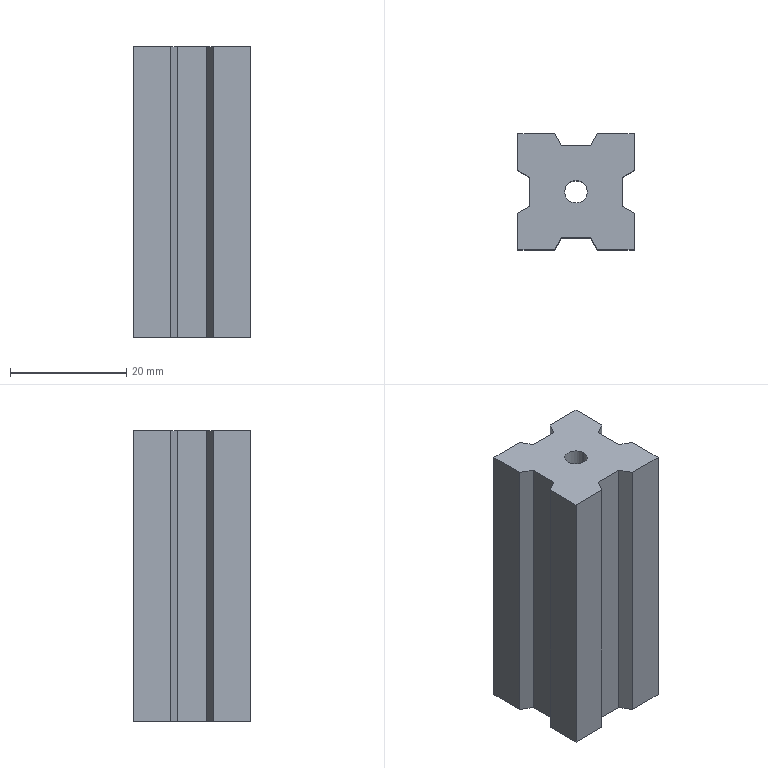Part | SolidWorks | features CirPattern 1, Extrusion 1, ICE 1 | 1 solid | 24 faces | box 20 x 20 x 50 mm | volume 16843 mm3 | plane 22 | cylinder 2 | commonest cylinder face diameters 3.889 x2
STEP:
#1=CARTESIAN_POINT('',(-1.944,0.,25.));
#2=VERTEX_POINT('',#1);
#3=CARTESIAN_POINT('',(1.944,0.,25.));
#4=VERTEX_POINT('',#3);
#5=CARTESIAN_POINT('',(0.,0.,25.));
#6=DIRECTION('',(0.,0.,1.));
#7=DIRECTION('',(1.,0.,0.));
#8=AXIS2_PLACEMENT_3D('',#5,#6,#7);
#9=CIRCLE('',#8,1.944);
#10=EDGE_CURVE('',#2,#4,#9,.T.);
#11=ORIENTED_EDGE('',*,*,#10,.T.);
#12=CARTESIAN_POINT('',(1.944,0.,-25.));
#13=VERTEX_POINT('',#12);
#14=CARTESIAN_POINT('',(1.944,0.,25.));
#15=DIRECTION('',(0.,0.,-1.));
#16=VECTOR('',#15,1000.);
#17=LINE('',#14,#16);
#18=EDGE_CURVE('',#4,#13,#17,.T.);
#19=ORIENTED_EDGE('',*,*,#18,.T.);
#20=CARTESIAN_POINT('',(-1.944,0.,-25.));
#21=VERTEX_POINT('',#20);
#22=CARTESIAN_POINT('',(0.,0.,-25.));
#23=DIRECTION('',(0.,0.,1.));
#24=DIRECTION('',(1.,0.,0.));
#25=AXIS2_PLACEMENT_3D('',#22,#23,#24);
#26=CIRCLE('',#25,1.944);
#27=EDGE_CURVE('',#21,#13,#26,.T.);
#28=ORIENTED_EDGE('',*,*,#27,.F.);
#29=CARTESIAN_POINT('',(-1.944,0.,25.));
#30=DIRECTION('',(0.,0.,-1.));
#31=VECTOR('',#30,1000.);
#32=LINE('',#29,#31);
#33=EDGE_CURVE('',#2,#21,#32,.T.);
#34=ORIENTED_EDGE('',*,*,#33,.F.);
#35=EDGE_LOOP('',(#11,#19,#28,#34));
#36=FACE_OUTER_BOUND('',#35,.T.);
#37=CARTESIAN_POINT('',(0.,0.,25.));
#38=DIRECTION('',(0.,0.,-1.));
#39=DIRECTION('',(-1.,0.,0.));
#40=AXIS2_PLACEMENT_3D('',#37,#38,#39);
#41=CYLINDRICAL_SURFACE('',#40,1.944);
#42=ADVANCED_FACE('',(#36),#41,.F.);
#43=CARTESIAN_POINT('',(-10.,3.694,25.));
#44=VERTEX_POINT('',#43);
#45=CARTESIAN_POINT('',(-10.,3.694,-25.));
#46=VERTEX_POINT('',#45);
#47=CARTESIAN_POINT('',(-10.,3.694,96.807));
#48=DIRECTION('',(0.,0.,-1.));
#49=VECTOR('',#48,1000.);
#50=LINE('',#47,#49);
#51=EDGE_CURVE('',#44,#46,#50,.T.);
#52=ORIENTED_EDGE('',*,*,#51,.F.);
#53=CARTESIAN_POINT('',(-10.,10.,25.));
#54=VERTEX_POINT('',#53);
#55=CARTESIAN_POINT('',(-10.,-10.,25.));
#56=DIRECTION('',(0.,-1.,0.));
#57=VECTOR('',#56,1000.);
#58=LINE('',#55,#57);
#59=EDGE_CURVE('',#54,#44,#58,.T.);
#60=ORIENTED_EDGE('',*,*,#59,.F.);
#61=CARTESIAN_POINT('',(-10.,10.,-25.));
#62=VERTEX_POINT('',#61);
#63=CARTESIAN_POINT('',(-10.,10.,25.));
#64=DIRECTION('',(0.,0.,-1.));
#65=VECTOR('',#64,1000.);
#66=LINE('',#63,#65);
#67=EDGE_CURVE('',#54,#62,#66,.T.);
#68=ORIENTED_EDGE('',*,*,#67,.T.);
#69=CARTESIAN_POINT('',(-10.,-10.,-25.));
#70=DIRECTION('',(0.,-1.,0.));
#71=VECTOR('',#70,1000.);
#72=LINE('',#69,#71);
#73=EDGE_CURVE('',#62,#46,#72,.T.);
#74=ORIENTED_EDGE('',*,*,#73,.T.);
#75=EDGE_LOOP('',(#52,#60,#68,#74));
#76=FACE_OUTER_BOUND('',#75,.T.);
#77=CARTESIAN_POINT('',(-10.,-10.,25.));
#78=DIRECTION('',(1.,0.,0.));
#79=DIRECTION('',(0.,0.,-1.));
#80=AXIS2_PLACEMENT_3D('',#77,#78,#79);
#81=PLANE('',#80);
#82=ADVANCED_FACE('',(#76),#81,.F.);
#83=ORIENTED_EDGE('',*,*,#10,.F.);
#84=CARTESIAN_POINT('',(0.,0.,25.));
#85=DIRECTION('',(0.,0.,1.));
#86=DIRECTION('',(1.,0.,0.));
#87=AXIS2_PLACEMENT_3D('',#84,#85,#86);
#88=CIRCLE('',#87,1.944);
#89=EDGE_CURVE('',#4,#2,#88,.T.);
#90=ORIENTED_EDGE('',*,*,#89,.F.);
#91=EDGE_LOOP('',(#83,#90));
#92=FACE_BOUND('',#91,.T.);
#93=CARTESIAN_POINT('',(-7.931,2.5,25.));
#94=VERTEX_POINT('',#93);
#95=CARTESIAN_POINT('',(-7.931,-2.5,25.));
#96=VERTEX_POINT('',#95);
#97=CARTESIAN_POINT('',(-7.931,0.,25.));
#98=DIRECTION('',(0.,-1.,0.));
#99=VECTOR('',#98,1000.);
#100=LINE('',#97,#99);
#101=EDGE_CURVE('',#94,#96,#100,.T.);
#102=ORIENTED_EDGE('',*,*,#101,.T.);
#103=CARTESIAN_POINT('',(-10.,-3.694,25.));
#104=VERTEX_POINT('',#103);
#105=CARTESIAN_POINT('',(-0.9003,1.559,25.));
#106=DIRECTION('',(-0.866,-0.5,0.));
#107=VECTOR('',#106,1000.);
#108=LINE('',#105,#107);
#109=EDGE_CURVE('',#96,#104,#108,.T.);
#110=ORIENTED_EDGE('',*,*,#109,.T.);
#111=CARTESIAN_POINT('',(-10.,-10.,25.));
#112=VERTEX_POINT('',#111);
#113=CARTESIAN_POINT('',(-10.,-10.,25.));
#114=DIRECTION('',(0.,-1.,0.));
#115=VECTOR('',#114,1000.);
#116=LINE('',#113,#115);
#117=EDGE_CURVE('',#104,#112,#116,.T.);
#118=ORIENTED_EDGE('',*,*,#117,.T.);
#119=CARTESIAN_POINT('',(-3.694,-10.,25.));
#120=VERTEX_POINT('',#119);
#121=CARTESIAN_POINT('',(10.,-10.,25.));
#122=DIRECTION('',(1.,0.,0.));
#123=VECTOR('',#122,1000.);
#124=LINE('',#121,#123);
#125=EDGE_CURVE('',#112,#120,#124,.T.);
#126=ORIENTED_EDGE('',*,*,#125,.T.);
#127=CARTESIAN_POINT('',(-2.5,-7.931,25.));
#128=VERTEX_POINT('',#127);
#129=CARTESIAN_POINT('',(1.559,-0.9003,25.));
#130=DIRECTION('',(0.5,0.866,0.));
#131=VECTOR('',#130,1000.);
#132=LINE('',#129,#131);
#133=EDGE_CURVE('',#120,#128,#132,.T.);
#134=ORIENTED_EDGE('',*,*,#133,.T.);
#135=CARTESIAN_POINT('',(2.5,-7.931,25.));
#136=VERTEX_POINT('',#135);
#137=CARTESIAN_POINT('',(0.,-7.931,25.));
#138=DIRECTION('',(1.,0.,0.));
#139=VECTOR('',#138,1000.);
#140=LINE('',#137,#139);
#141=EDGE_CURVE('',#128,#136,#140,.T.);
#142=ORIENTED_EDGE('',*,*,#141,.T.);
#143=CARTESIAN_POINT('',(3.694,-10.,25.));
#144=VERTEX_POINT('',#143);
#145=CARTESIAN_POINT('',(-1.559,-0.9003,25.));
#146=DIRECTION('',(0.5,-0.866,0.));
#147=VECTOR('',#146,1000.);
#148=LINE('',#145,#147);
#149=EDGE_CURVE('',#136,#144,#148,.T.);
#150=ORIENTED_EDGE('',*,*,#149,.T.);
#151=CARTESIAN_POINT('',(10.,-10.,25.));
#152=VERTEX_POINT('',#151);
#153=CARTESIAN_POINT('',(10.,-10.,25.));
#154=DIRECTION('',(1.,0.,0.));
#155=VECTOR('',#154,1000.);
#156=LINE('',#153,#155);
#157=EDGE_CURVE('',#144,#152,#156,.T.);
#158=ORIENTED_EDGE('',*,*,#157,.T.);
#159=CARTESIAN_POINT('',(10.,-3.694,25.));
#160=VERTEX_POINT('',#159);
#161=CARTESIAN_POINT('',(10.,-10.,25.));
#162=DIRECTION('',(0.,1.,0.));
#163=VECTOR('',#162,1000.);
#164=LINE('',#161,#163);
#165=EDGE_CURVE('',#152,#160,#164,.T.);
#166=ORIENTED_EDGE('',*,*,#165,.T.);
#167=CARTESIAN_POINT('',(7.931,-2.5,25.));
#168=VERTEX_POINT('',#167);
#169=CARTESIAN_POINT('',(0.9003,1.559,25.));
#170=DIRECTION('',(-0.866,0.5,0.));
#171=VECTOR('',#170,1000.);
#172=LINE('',#169,#171);
#173=EDGE_CURVE('',#160,#168,#172,.T.);
#174=ORIENTED_EDGE('',*,*,#173,.T.);
#175=CARTESIAN_POINT('',(7.931,2.5,25.));
#176=VERTEX_POINT('',#175);
#177=CARTESIAN_POINT('',(7.931,0.,25.));
#178=DIRECTION('',(0.,1.,0.));
#179=VECTOR('',#178,1000.);
#180=LINE('',#177,#179);
#181=EDGE_CURVE('',#168,#176,#180,.T.);
#182=ORIENTED_EDGE('',*,*,#181,.T.);
#183=CARTESIAN_POINT('',(10.,3.694,25.));
#184=VERTEX_POINT('',#183);
#185=CARTESIAN_POINT('',(0.9003,-1.559,25.));
#186=DIRECTION('',(0.866,0.5,0.));
#187=VECTOR('',#186,1000.);
#188=LINE('',#185,#187);
#189=EDGE_CURVE('',#176,#184,#188,.T.);
#190=ORIENTED_EDGE('',*,*,#189,.T.);
#191=CARTESIAN_POINT('',(10.,10.,25.));
#192=VERTEX_POINT('',#191);
#193=CARTESIAN_POINT('',(10.,-10.,25.));
#194=DIRECTION('',(0.,1.,0.));
#195=VECTOR('',#194,1000.);
#196=LINE('',#193,#195);
#197=EDGE_CURVE('',#184,#192,#196,.T.);
#198=ORIENTED_EDGE('',*,*,#197,.T.);
#199=CARTESIAN_POINT('',(3.694,10.,25.));
#200=VERTEX_POINT('',#199);
#201=CARTESIAN_POINT('',(10.,10.,25.));
#202=DIRECTION('',(-1.,0.,0.));
#203=VECTOR('',#202,1000.);
#204=LINE('',#201,#203);
#205=EDGE_CURVE('',#192,#200,#204,.T.);
#206=ORIENTED_EDGE('',*,*,#205,.T.);
#207=CARTESIAN_POINT('',(2.5,7.931,25.));
#208=VERTEX_POINT('',#207);
#209=CARTESIAN_POINT('',(-1.559,0.9003,25.));
#210=DIRECTION('',(-0.5,-0.866,0.));
#211=VECTOR('',#210,1000.);
#212=LINE('',#209,#211);
#213=EDGE_CURVE('',#200,#208,#212,.T.);
#214=ORIENTED_EDGE('',*,*,#213,.T.);
#215=CARTESIAN_POINT('',(-2.5,7.931,25.));
#216=VERTEX_POINT('',#215);
#217=CARTESIAN_POINT('',(0.,7.931,25.));
#218=DIRECTION('',(-1.,0.,0.));
#219=VECTOR('',#218,1000.);
#220=LINE('',#217,#219);
#221=EDGE_CURVE('',#208,#216,#220,.T.);
#222=ORIENTED_EDGE('',*,*,#221,.T.);
#223=CARTESIAN_POINT('',(-3.694,10.,25.));
#224=VERTEX_POINT('',#223);
#225=CARTESIAN_POINT('',(1.559,0.9003,25.));
#226=DIRECTION('',(-0.5,0.866,0.));
#227=VECTOR('',#226,1000.);
#228=LINE('',#225,#227);
#229=EDGE_CURVE('',#216,#224,#228,.T.);
#230=ORIENTED_EDGE('',*,*,#229,.T.);
#231=CARTESIAN_POINT('',(10.,10.,25.));
#232=DIRECTION('',(-1.,0.,0.));
#233=VECTOR('',#232,1000.);
#234=LINE('',#231,#233);
#235=EDGE_CURVE('',#224,#54,#234,.T.);
#236=ORIENTED_EDGE('',*,*,#235,.T.);
#237=ORIENTED_EDGE('',*,*,#59,.T.);
#238=CARTESIAN_POINT('',(-0.9003,-1.559,25.));
#239=DIRECTION('',(0.866,-0.5,0.));
#240=VECTOR('',#239,1000.);
#241=LINE('',#238,#240);
#242=EDGE_CURVE('',#44,#94,#241,.T.);
#243=ORIENTED_EDGE('',*,*,#242,.T.);
#244=EDGE_LOOP('',(#102,#110,#118,#126,#134,#142,#150,#158,#166,#174,#182,#190,#198,#206,#214,#222,#230,#236,#237,#243));
#245=FACE_OUTER_BOUND('',#244,.T.);
#246=CARTESIAN_POINT('',(0.,0.,25.));
#247=DIRECTION('',(0.,0.,1.));
#248=DIRECTION('',(1.,0.,0.));
#249=AXIS2_PLACEMENT_3D('',#246,#247,#248);
#250=PLANE('',#249);
#251=ADVANCED_FACE('',(#92,#245),#250,.T.);
#252=ORIENTED_EDGE('',*,*,#27,.T.);
#253=CARTESIAN_POINT('',(0.,0.,-25.));
#254=DIRECTION('',(0.,0.,1.));
#255=DIRECTION('',(1.,0.,0.));
#256=AXIS2_PLACEMENT_3D('',#253,#254,#255);
#257=CIRCLE('',#256,1.944);
#258=EDGE_CURVE('',#13,#21,#257,.T.);
#259=ORIENTED_EDGE('',*,*,#258,.T.);
#260=EDGE_LOOP('',(#252,#259));
#261=FACE_BOUND('',#260,.T.);
#262=CARTESIAN_POINT('',(-7.931,-2.5,-25.));
#263=VERTEX_POINT('',#262);
#264=CARTESIAN_POINT('',(-10.,-3.694,-25.));
#265=VERTEX_POINT('',#264);
#266=CARTESIAN_POINT('',(-0.9003,1.559,-25.));
#267=DIRECTION('',(-0.866,-0.5,0.));
#268=VECTOR('',#267,1000.);
#269=LINE('',#266,#268);
#270=EDGE_CURVE('',#263,#265,#269,.T.);
#271=ORIENTED_EDGE('',*,*,#270,.F.);
#272=CARTESIAN_POINT('',(-7.931,2.5,-25.));
#273=VERTEX_POINT('',#272);
#274=CARTESIAN_POINT('',(-7.931,0.,-25.));
#275=DIRECTION('',(0.,-1.,0.));
#276=VECTOR('',#275,1000.);
#277=LINE('',#274,#276);
#278=EDGE_CURVE('',#273,#263,#277,.T.);
#279=ORIENTED_EDGE('',*,*,#278,.F.);
#280=CARTESIAN_POINT('',(-0.9003,-1.559,-25.));
#281=DIRECTION('',(0.866,-0.5,0.));
#282=VECTOR('',#281,1000.);
#283=LINE('',#280,#282);
#284=EDGE_CURVE('',#46,#273,#283,.T.);
#285=ORIENTED_EDGE('',*,*,#284,.F.);
#286=ORIENTED_EDGE('',*,*,#73,.F.);
#287=CARTESIAN_POINT('',(-3.694,10.,-25.));
#288=VERTEX_POINT('',#287);
#289=CARTESIAN_POINT('',(10.,10.,-25.));
#290=DIRECTION('',(-1.,0.,0.));
#291=VECTOR('',#290,1000.);
#292=LINE('',#289,#291);
#293=EDGE_CURVE('',#288,#62,#292,.T.);
#294=ORIENTED_EDGE('',*,*,#293,.F.);
#295=CARTESIAN_POINT('',(-2.5,7.931,-25.));
#296=VERTEX_POINT('',#295);
#297=CARTESIAN_POINT('',(1.559,0.9003,-25.));
#298=DIRECTION('',(-0.5,0.866,0.));
#299=VECTOR('',#298,1000.);
#300=LINE('',#297,#299);
#301=EDGE_CURVE('',#296,#288,#300,.T.);
#302=ORIENTED_EDGE('',*,*,#301,.F.);
#303=CARTESIAN_POINT('',(2.5,7.931,-25.));
#304=VERTEX_POINT('',#303);
#305=CARTESIAN_POINT('',(0.,7.931,-25.));
#306=DIRECTION('',(-1.,0.,0.));
#307=VECTOR('',#306,1000.);
#308=LINE('',#305,#307);
#309=EDGE_CURVE('',#304,#296,#308,.T.);
#310=ORIENTED_EDGE('',*,*,#309,.F.);
#311=CARTESIAN_POINT('',(3.694,10.,-25.));
#312=VERTEX_POINT('',#311);
#313=CARTESIAN_POINT('',(-1.559,0.9003,-25.));
#314=DIRECTION('',(-0.5,-0.866,0.));
#315=VECTOR('',#314,1000.);
#316=LINE('',#313,#315);
#317=EDGE_CURVE('',#312,#304,#316,.T.);
#318=ORIENTED_EDGE('',*,*,#317,.F.);
#319=CARTESIAN_POINT('',(10.,10.,-25.));
#320=VERTEX_POINT('',#319);
#321=CARTESIAN_POINT('',(10.,10.,-25.));
#322=DIRECTION('',(-1.,0.,0.));
#323=VECTOR('',#322,1000.);
#324=LINE('',#321,#323);
#325=EDGE_CURVE('',#320,#312,#324,.T.);
#326=ORIENTED_EDGE('',*,*,#325,.F.);
#327=CARTESIAN_POINT('',(10.,3.694,-25.));
#328=VERTEX_POINT('',#327);
#329=CARTESIAN_POINT('',(10.,-10.,-25.));
#330=DIRECTION('',(0.,1.,0.));
#331=VECTOR('',#330,1000.);
#332=LINE('',#329,#331);
#333=EDGE_CURVE('',#328,#320,#332,.T.);
#334=ORIENTED_EDGE('',*,*,#333,.F.);
#335=CARTESIAN_POINT('',(7.931,2.5,-25.));
#336=VERTEX_POINT('',#335);
#337=CARTESIAN_POINT('',(0.9003,-1.559,-25.));
#338=DIRECTION('',(0.866,0.5,0.));
#339=VECTOR('',#338,1000.);
#340=LINE('',#337,#339);
#341=EDGE_CURVE('',#336,#328,#340,.T.);
#342=ORIENTED_EDGE('',*,*,#341,.F.);
#343=CARTESIAN_POINT('',(7.931,-2.5,-25.));
#344=VERTEX_POINT('',#343);
#345=CARTESIAN_POINT('',(7.931,0.,-25.));
#346=DIRECTION('',(0.,1.,0.));
#347=VECTOR('',#346,1000.);
#348=LINE('',#345,#347);
#349=EDGE_CURVE('',#344,#336,#348,.T.);
#350=ORIENTED_EDGE('',*,*,#349,.F.);
#351=CARTESIAN_POINT('',(10.,-3.694,-25.));
#352=VERTEX_POINT('',#351);
#353=CARTESIAN_POINT('',(0.9003,1.559,-25.));
#354=DIRECTION('',(-0.866,0.5,0.));
#355=VECTOR('',#354,1000.);
#356=LINE('',#353,#355);
#357=EDGE_CURVE('',#352,#344,#356,.T.);
#358=ORIENTED_EDGE('',*,*,#357,.F.);
#359=CARTESIAN_POINT('',(10.,-10.,-25.));
#360=VERTEX_POINT('',#359);
#361=CARTESIAN_POINT('',(10.,-10.,-25.));
#362=DIRECTION('',(0.,1.,0.));
#363=VECTOR('',#362,1000.);
#364=LINE('',#361,#363);
#365=EDGE_CURVE('',#360,#352,#364,.T.);
#366=ORIENTED_EDGE('',*,*,#365,.F.);
#367=CARTESIAN_POINT('',(3.694,-10.,-25.));
#368=VERTEX_POINT('',#367);
#369=CARTESIAN_POINT('',(10.,-10.,-25.));
#370=DIRECTION('',(1.,0.,0.));
#371=VECTOR('',#370,1000.);
#372=LINE('',#369,#371);
#373=EDGE_CURVE('',#368,#360,#372,.T.);
#374=ORIENTED_EDGE('',*,*,#373,.F.);
#375=CARTESIAN_POINT('',(2.5,-7.931,-25.));
#376=VERTEX_POINT('',#375);
#377=CARTESIAN_POINT('',(-1.559,-0.9003,-25.));
#378=DIRECTION('',(0.5,-0.866,0.));
#379=VECTOR('',#378,1000.);
#380=LINE('',#377,#379);
#381=EDGE_CURVE('',#376,#368,#380,.T.);
#382=ORIENTED_EDGE('',*,*,#381,.F.);
#383=CARTESIAN_POINT('',(-2.5,-7.931,-25.));
#384=VERTEX_POINT('',#383);
#385=CARTESIAN_POINT('',(0.,-7.931,-25.));
#386=DIRECTION('',(1.,0.,0.));
#387=VECTOR('',#386,1000.);
#388=LINE('',#385,#387);
#389=EDGE_CURVE('',#384,#376,#388,.T.);
#390=ORIENTED_EDGE('',*,*,#389,.F.);
#391=CARTESIAN_POINT('',(-3.694,-10.,-25.));
#392=VERTEX_POINT('',#391);
#393=CARTESIAN_POINT('',(1.559,-0.9003,-25.));
#394=DIRECTION('',(0.5,0.866,0.));
#395=VECTOR('',#394,1000.);
#396=LINE('',#393,#395);
#397=EDGE_CURVE('',#392,#384,#396,.T.);
#398=ORIENTED_EDGE('',*,*,#397,.F.);
#399=CARTESIAN_POINT('',(-10.,-10.,-25.));
#400=VERTEX_POINT('',#399);
#401=CARTESIAN_POINT('',(10.,-10.,-25.));
#402=DIRECTION('',(1.,0.,0.));
#403=VECTOR('',#402,1000.);
#404=LINE('',#401,#403);
#405=EDGE_CURVE('',#400,#392,#404,.T.);
#406=ORIENTED_EDGE('',*,*,#405,.F.);
#407=CARTESIAN_POINT('',(-10.,-10.,-25.));
#408=DIRECTION('',(0.,-1.,0.));
#409=VECTOR('',#408,1000.);
#410=LINE('',#407,#409);
#411=EDGE_CURVE('',#265,#400,#410,.T.);
#412=ORIENTED_EDGE('',*,*,#411,.F.);
#413=EDGE_LOOP('',(#271,#279,#285,#286,#294,#302,#310,#318,#326,#334,#342,#350,#358,#366,#374,#382,#390,#398,#406,#412));
#414=FACE_OUTER_BOUND('',#413,.T.);
#415=CARTESIAN_POINT('',(0.,0.,-25.));
#416=DIRECTION('',(0.,0.,1.));
#417=DIRECTION('',(1.,0.,0.));
#418=AXIS2_PLACEMENT_3D('',#415,#416,#417);
#419=PLANE('',#418);
#420=ADVANCED_FACE('',(#261,#414),#419,.F.);
#421=CARTESIAN_POINT('',(-3.694,-10.,96.807));
#422=DIRECTION('',(0.,0.,-1.));
#423=VECTOR('',#422,1000.);
#424=LINE('',#421,#423);
#425=EDGE_CURVE('',#120,#392,#424,.T.);
#426=ORIENTED_EDGE('',*,*,#425,.F.);
#427=ORIENTED_EDGE('',*,*,#125,.F.);
#428=CARTESIAN_POINT('',(-10.,-10.,25.));
#429=DIRECTION('',(0.,0.,-1.));
#430=VECTOR('',#429,1000.);
#431=LINE('',#428,#430);
#432=EDGE_CURVE('',#112,#400,#431,.T.);
#433=ORIENTED_EDGE('',*,*,#432,.T.);
#434=ORIENTED_EDGE('',*,*,#405,.T.);
#435=EDGE_LOOP('',(#426,#427,#433,#434));
#436=FACE_OUTER_BOUND('',#435,.T.);
#437=CARTESIAN_POINT('',(10.,-10.,25.));
#438=DIRECTION('',(0.,1.,0.));
#439=DIRECTION('',(-1.,0.,0.));
#440=AXIS2_PLACEMENT_3D('',#437,#438,#439);
#441=PLANE('',#440);
#442=ADVANCED_FACE('',(#436),#441,.F.);
#443=CARTESIAN_POINT('',(10.,-3.694,96.807));
#444=DIRECTION('',(0.,0.,-1.));
#445=VECTOR('',#444,1000.);
#446=LINE('',#443,#445);
#447=EDGE_CURVE('',#160,#352,#446,.T.);
#448=ORIENTED_EDGE('',*,*,#447,.F.);
#449=ORIENTED_EDGE('',*,*,#165,.F.);
#450=CARTESIAN_POINT('',(10.,-10.,25.));
#451=DIRECTION('',(0.,0.,-1.));
#452=VECTOR('',#451,1000.);
#453=LINE('',#450,#452);
#454=EDGE_CURVE('',#152,#360,#453,.T.);
#455=ORIENTED_EDGE('',*,*,#454,.T.);
#456=ORIENTED_EDGE('',*,*,#365,.T.);
#457=EDGE_LOOP('',(#448,#449,#455,#456));
#458=FACE_OUTER_BOUND('',#457,.T.);
#459=CARTESIAN_POINT('',(10.,-10.,25.));
#460=DIRECTION('',(-1.,0.,0.));
#461=DIRECTION('',(0.,0.,1.));
#462=AXIS2_PLACEMENT_3D('',#459,#460,#461);
#463=PLANE('',#462);
#464=ADVANCED_FACE('',(#458),#463,.F.);
#465=CARTESIAN_POINT('',(3.694,10.,96.807));
#466=DIRECTION('',(0.,0.,-1.));
#467=VECTOR('',#466,1000.);
#468=LINE('',#465,#467);
#469=EDGE_CURVE('',#200,#312,#468,.T.);
#470=ORIENTED_EDGE('',*,*,#469,.F.);
#471=ORIENTED_EDGE('',*,*,#205,.F.);
#472=CARTESIAN_POINT('',(10.,10.,25.));
#473=DIRECTION('',(0.,0.,-1.));
#474=VECTOR('',#473,1000.);
#475=LINE('',#472,#474);
#476=EDGE_CURVE('',#192,#320,#475,.T.);
#477=ORIENTED_EDGE('',*,*,#476,.T.);
#478=ORIENTED_EDGE('',*,*,#325,.T.);
#479=EDGE_LOOP('',(#470,#471,#477,#478));
#480=FACE_OUTER_BOUND('',#479,.T.);
#481=CARTESIAN_POINT('',(10.,10.,25.));
#482=DIRECTION('',(0.,-1.,0.));
#483=DIRECTION('',(1.,0.,0.));
#484=AXIS2_PLACEMENT_3D('',#481,#482,#483);
#485=PLANE('',#484);
#486=ADVANCED_FACE('',(#480),#485,.F.);
#487=ORIENTED_EDGE('',*,*,#117,.F.);
#488=CARTESIAN_POINT('',(-10.,-3.694,96.807));
#489=DIRECTION('',(0.,0.,-1.));
#490=VECTOR('',#489,1000.);
#491=LINE('',#488,#490);
#492=EDGE_CURVE('',#104,#265,#491,.T.);
#493=ORIENTED_EDGE('',*,*,#492,.T.);
#494=ORIENTED_EDGE('',*,*,#411,.T.);
#495=ORIENTED_EDGE('',*,*,#432,.F.);
#496=EDGE_LOOP('',(#487,#493,#494,#495));
#497=FACE_OUTER_BOUND('',#496,.T.);
#498=CARTESIAN_POINT('',(-10.,-10.,25.));
#499=DIRECTION('',(1.,0.,0.));
#500=DIRECTION('',(0.,0.,-1.));
#501=AXIS2_PLACEMENT_3D('',#498,#499,#500);
#502=PLANE('',#501);
#503=ADVANCED_FACE('',(#497),#502,.F.);
#504=ORIENTED_EDGE('',*,*,#157,.F.);
#505=CARTESIAN_POINT('',(3.694,-10.,96.807));
#506=DIRECTION('',(0.,0.,-1.));
#507=VECTOR('',#506,1000.);
#508=LINE('',#505,#507);
#509=EDGE_CURVE('',#144,#368,#508,.T.);
#510=ORIENTED_EDGE('',*,*,#509,.T.);
#511=ORIENTED_EDGE('',*,*,#373,.T.);
#512=ORIENTED_EDGE('',*,*,#454,.F.);
#513=EDGE_LOOP('',(#504,#510,#511,#512));
#514=FACE_OUTER_BOUND('',#513,.T.);
#515=CARTESIAN_POINT('',(10.,-10.,25.));
#516=DIRECTION('',(0.,1.,0.));
#517=DIRECTION('',(-1.,0.,0.));
#518=AXIS2_PLACEMENT_3D('',#515,#516,#517);
#519=PLANE('',#518);
#520=ADVANCED_FACE('',(#514),#519,.F.);
#521=ORIENTED_EDGE('',*,*,#197,.F.);
#522=CARTESIAN_POINT('',(10.,3.694,96.807));
#523=DIRECTION('',(0.,0.,-1.));
#524=VECTOR('',#523,1000.);
#525=LINE('',#522,#524);
#526=EDGE_CURVE('',#184,#328,#525,.T.);
#527=ORIENTED_EDGE('',*,*,#526,.T.);
#528=ORIENTED_EDGE('',*,*,#333,.T.);
#529=ORIENTED_EDGE('',*,*,#476,.F.);
#530=EDGE_LOOP('',(#521,#527,#528,#529));
#531=FACE_OUTER_BOUND('',#530,.T.);
#532=CARTESIAN_POINT('',(10.,-10.,25.));
#533=DIRECTION('',(-1.,0.,0.));
#534=DIRECTION('',(0.,0.,1.));
#535=AXIS2_PLACEMENT_3D('',#532,#533,#534);
#536=PLANE('',#535);
#537=ADVANCED_FACE('',(#531),#536,.F.);
#538=ORIENTED_EDGE('',*,*,#235,.F.);
#539=CARTESIAN_POINT('',(-3.694,10.,96.807));
#540=DIRECTION('',(0.,0.,-1.));
#541=VECTOR('',#540,1000.);
#542=LINE('',#539,#541);
#543=EDGE_CURVE('',#224,#288,#542,.T.);
#544=ORIENTED_EDGE('',*,*,#543,.T.);
#545=ORIENTED_EDGE('',*,*,#293,.T.);
#546=ORIENTED_EDGE('',*,*,#67,.F.);
#547=EDGE_LOOP('',(#538,#544,#545,#546));
#548=FACE_OUTER_BOUND('',#547,.T.);
#549=CARTESIAN_POINT('',(10.,10.,25.));
#550=DIRECTION('',(0.,-1.,0.));
#551=DIRECTION('',(1.,0.,0.));
#552=AXIS2_PLACEMENT_3D('',#549,#550,#551);
#553=PLANE('',#552);
#554=ADVANCED_FACE('',(#548),#553,.F.);
#555=ORIENTED_EDGE('',*,*,#18,.F.);
#556=ORIENTED_EDGE('',*,*,#89,.T.);
#557=ORIENTED_EDGE('',*,*,#33,.T.);
#558=ORIENTED_EDGE('',*,*,#258,.F.);
#559=EDGE_LOOP('',(#555,#556,#557,#558));
#560=FACE_OUTER_BOUND('',#559,.T.);
#561=CARTESIAN_POINT('',(0.,0.,25.));
#562=DIRECTION('',(0.,0.,-1.));
#563=DIRECTION('',(-1.,0.,0.));
#564=AXIS2_PLACEMENT_3D('',#561,#562,#563);
#565=CYLINDRICAL_SURFACE('',#564,1.944);
#566=ADVANCED_FACE('',(#560),#565,.F.);
#567=ORIENTED_EDGE('',*,*,#229,.F.);
#568=CARTESIAN_POINT('',(-2.5,7.931,96.807));
#569=DIRECTION('',(0.,0.,-1.));
#570=VECTOR('',#569,1000.);
#571=LINE('',#568,#570);
#572=EDGE_CURVE('',#216,#296,#571,.T.);
#573=ORIENTED_EDGE('',*,*,#572,.T.);
#574=ORIENTED_EDGE('',*,*,#301,.T.);
#575=ORIENTED_EDGE('',*,*,#543,.F.);
#576=EDGE_LOOP('',(#567,#573,#574,#575));
#577=FACE_OUTER_BOUND('',#576,.T.);
#578=CARTESIAN_POINT('',(-3.694,10.,96.807));
#579=DIRECTION('',(0.866,0.5,0.));
#580=DIRECTION('',(-0.5,0.866,0.));
#581=AXIS2_PLACEMENT_3D('',#578,#579,#580);
#582=PLANE('',#581);
#583=ADVANCED_FACE('',(#577),#582,.T.);
#584=ORIENTED_EDGE('',*,*,#221,.F.);
#585=CARTESIAN_POINT('',(2.5,7.931,96.807));
#586=DIRECTION('',(0.,0.,-1.));
#587=VECTOR('',#586,1000.);
#588=LINE('',#585,#587);
#589=EDGE_CURVE('',#208,#304,#588,.T.);
#590=ORIENTED_EDGE('',*,*,#589,.T.);
#591=ORIENTED_EDGE('',*,*,#309,.T.);
#592=ORIENTED_EDGE('',*,*,#572,.F.);
#593=EDGE_LOOP('',(#584,#590,#591,#592));
#594=FACE_OUTER_BOUND('',#593,.T.);
#595=CARTESIAN_POINT('',(-2.5,7.931,96.807));
#596=DIRECTION('',(0.,1.,0.));
#597=DIRECTION('',(0.,0.,1.));
#598=AXIS2_PLACEMENT_3D('',#595,#596,#597);
#599=PLANE('',#598);
#600=ADVANCED_FACE('',(#594),#599,.T.);
#601=ORIENTED_EDGE('',*,*,#213,.F.);
#602=ORIENTED_EDGE('',*,*,#469,.T.);
#603=ORIENTED_EDGE('',*,*,#317,.T.);
#604=ORIENTED_EDGE('',*,*,#589,.F.);
#605=EDGE_LOOP('',(#601,#602,#603,#604));
#606=FACE_OUTER_BOUND('',#605,.T.);
#607=CARTESIAN_POINT('',(2.5,7.931,96.807));
#608=DIRECTION('',(-0.866,0.5,0.));
#609=DIRECTION('',(-0.5,-0.866,0.));
#610=AXIS2_PLACEMENT_3D('',#607,#608,#609);
#611=PLANE('',#610);
#612=ADVANCED_FACE('',(#606),#611,.T.);
#613=ORIENTED_EDGE('',*,*,#189,.F.);
#614=CARTESIAN_POINT('',(7.931,2.5,96.807));
#615=DIRECTION('',(0.,0.,-1.));
#616=VECTOR('',#615,1000.);
#617=LINE('',#614,#616);
#618=EDGE_CURVE('',#176,#336,#617,.T.);
#619=ORIENTED_EDGE('',*,*,#618,.T.);
#620=ORIENTED_EDGE('',*,*,#341,.T.);
#621=ORIENTED_EDGE('',*,*,#526,.F.);
#622=EDGE_LOOP('',(#613,#619,#620,#621));
#623=FACE_OUTER_BOUND('',#622,.T.);
#624=CARTESIAN_POINT('',(10.,3.694,96.807));
#625=DIRECTION('',(0.5,-0.866,0.));
#626=DIRECTION('',(0.866,0.5,0.));
#627=AXIS2_PLACEMENT_3D('',#624,#625,#626);
#628=PLANE('',#627);
#629=ADVANCED_FACE('',(#623),#628,.T.);
#630=ORIENTED_EDGE('',*,*,#181,.F.);
#631=CARTESIAN_POINT('',(7.931,-2.5,96.807));
#632=DIRECTION('',(0.,0.,-1.));
#633=VECTOR('',#632,1000.);
#634=LINE('',#631,#633);
#635=EDGE_CURVE('',#168,#344,#634,.T.);
#636=ORIENTED_EDGE('',*,*,#635,.T.);
#637=ORIENTED_EDGE('',*,*,#349,.T.);
#638=ORIENTED_EDGE('',*,*,#618,.F.);
#639=EDGE_LOOP('',(#630,#636,#637,#638));
#640=FACE_OUTER_BOUND('',#639,.T.);
#641=CARTESIAN_POINT('',(7.931,2.5,96.807));
#642=DIRECTION('',(1.,0.,0.));
#643=DIRECTION('',(0.,1.,0.));
#644=AXIS2_PLACEMENT_3D('',#641,#642,#643);
#645=PLANE('',#644);
#646=ADVANCED_FACE('',(#640),#645,.T.);
#647=ORIENTED_EDGE('',*,*,#173,.F.);
#648=ORIENTED_EDGE('',*,*,#447,.T.);
#649=ORIENTED_EDGE('',*,*,#357,.T.);
#650=ORIENTED_EDGE('',*,*,#635,.F.);
#651=EDGE_LOOP('',(#647,#648,#649,#650));
#652=FACE_OUTER_BOUND('',#651,.T.);
#653=CARTESIAN_POINT('',(7.931,-2.5,96.807));
#654=DIRECTION('',(0.5,0.866,0.));
#655=DIRECTION('',(-0.866,0.5,0.));
#656=AXIS2_PLACEMENT_3D('',#653,#654,#655);
#657=PLANE('',#656);
#658=ADVANCED_FACE('',(#652),#657,.T.);
#659=ORIENTED_EDGE('',*,*,#149,.F.);
#660=CARTESIAN_POINT('',(2.5,-7.931,96.807));
#661=DIRECTION('',(0.,0.,-1.));
#662=VECTOR('',#661,1000.);
#663=LINE('',#660,#662);
#664=EDGE_CURVE('',#136,#376,#663,.T.);
#665=ORIENTED_EDGE('',*,*,#664,.T.);
#666=ORIENTED_EDGE('',*,*,#381,.T.);
#667=ORIENTED_EDGE('',*,*,#509,.F.);
#668=EDGE_LOOP('',(#659,#665,#666,#667));
#669=FACE_OUTER_BOUND('',#668,.T.);
#670=CARTESIAN_POINT('',(3.694,-10.,96.807));
#671=DIRECTION('',(-0.866,-0.5,0.));
#672=DIRECTION('',(0.5,-0.866,0.));
#673=AXIS2_PLACEMENT_3D('',#670,#671,#672);
#674=PLANE('',#673);
#675=ADVANCED_FACE('',(#669),#674,.T.);
#676=ORIENTED_EDGE('',*,*,#141,.F.);
#677=CARTESIAN_POINT('',(-2.5,-7.931,96.807));
#678=DIRECTION('',(0.,0.,-1.));
#679=VECTOR('',#678,1000.);
#680=LINE('',#677,#679);
#681=EDGE_CURVE('',#128,#384,#680,.T.);
#682=ORIENTED_EDGE('',*,*,#681,.T.);
#683=ORIENTED_EDGE('',*,*,#389,.T.);
#684=ORIENTED_EDGE('',*,*,#664,.F.);
#685=EDGE_LOOP('',(#676,#682,#683,#684));
#686=FACE_OUTER_BOUND('',#685,.T.);
#687=CARTESIAN_POINT('',(2.5,-7.931,96.807));
#688=DIRECTION('',(0.,-1.,0.));
#689=DIRECTION('',(0.,0.,-1.));
#690=AXIS2_PLACEMENT_3D('',#687,#688,#689);
#691=PLANE('',#690);
#692=ADVANCED_FACE('',(#686),#691,.T.);
#693=ORIENTED_EDGE('',*,*,#133,.F.);
#694=ORIENTED_EDGE('',*,*,#425,.T.);
#695=ORIENTED_EDGE('',*,*,#397,.T.);
#696=ORIENTED_EDGE('',*,*,#681,.F.);
#697=EDGE_LOOP('',(#693,#694,#695,#696));
#698=FACE_OUTER_BOUND('',#697,.T.);
#699=CARTESIAN_POINT('',(-2.5,-7.931,96.807));
#700=DIRECTION('',(0.866,-0.5,0.));
#701=DIRECTION('',(0.5,0.866,0.));
#702=AXIS2_PLACEMENT_3D('',#699,#700,#701);
#703=PLANE('',#702);
#704=ADVANCED_FACE('',(#698),#703,.T.);
#705=ORIENTED_EDGE('',*,*,#109,.F.);
#706=CARTESIAN_POINT('',(-7.931,-2.5,96.807));
#707=DIRECTION('',(0.,0.,-1.));
#708=VECTOR('',#707,1000.);
#709=LINE('',#706,#708);
#710=EDGE_CURVE('',#96,#263,#709,.T.);
#711=ORIENTED_EDGE('',*,*,#710,.T.);
#712=ORIENTED_EDGE('',*,*,#270,.T.);
#713=ORIENTED_EDGE('',*,*,#492,.F.);
#714=EDGE_LOOP('',(#705,#711,#712,#713));
#715=FACE_OUTER_BOUND('',#714,.T.);
#716=CARTESIAN_POINT('',(-10.,-3.694,96.807));
#717=DIRECTION('',(-0.5,0.866,0.));
#718=DIRECTION('',(-0.866,-0.5,0.));
#719=AXIS2_PLACEMENT_3D('',#716,#717,#718);
#720=PLANE('',#719);
#721=ADVANCED_FACE('',(#715),#720,.T.);
#722=ORIENTED_EDGE('',*,*,#101,.F.);
#723=CARTESIAN_POINT('',(-7.931,2.5,96.807));
#724=DIRECTION('',(0.,0.,-1.));
#725=VECTOR('',#724,1000.);
#726=LINE('',#723,#725);
#727=EDGE_CURVE('',#94,#273,#726,.T.);
#728=ORIENTED_EDGE('',*,*,#727,.T.);
#729=ORIENTED_EDGE('',*,*,#278,.T.);
#730=ORIENTED_EDGE('',*,*,#710,.F.);
#731=EDGE_LOOP('',(#722,#728,#729,#730));
#732=FACE_OUTER_BOUND('',#731,.T.);
#733=CARTESIAN_POINT('',(-7.931,-2.5,96.807));
#734=DIRECTION('',(-1.,0.,0.));
#735=DIRECTION('',(0.,-1.,0.));
#736=AXIS2_PLACEMENT_3D('',#733,#734,#735);
#737=PLANE('',#736);
#738=ADVANCED_FACE('',(#732),#737,.T.);
#739=ORIENTED_EDGE('',*,*,#242,.F.);
#740=ORIENTED_EDGE('',*,*,#51,.T.);
#741=ORIENTED_EDGE('',*,*,#284,.T.);
#742=ORIENTED_EDGE('',*,*,#727,.F.);
#743=EDGE_LOOP('',(#739,#740,#741,#742));
#744=FACE_OUTER_BOUND('',#743,.T.);
#745=CARTESIAN_POINT('',(-7.931,2.5,96.807));
#746=DIRECTION('',(-0.5,-0.866,0.));
#747=DIRECTION('',(0.866,-0.5,0.));
#748=AXIS2_PLACEMENT_3D('',#745,#746,#747);
#749=PLANE('',#748);
#750=ADVANCED_FACE('',(#744),#749,.T.);
#751=CLOSED_SHELL('',(#42,#82,#251,#420,#442,#464,#486,#503,#520,#537,#554,#566,#583,#600,#612,#629,#646,#658,#675,#692,#704,#721,#738,#750));
#752=MANIFOLD_SOLID_BREP('',#751);
#753=CARTESIAN_POINT('',(0.,0.,0.));
#754=DIRECTION('',(0.,0.,1.));
#755=DIRECTION('',(1.,0.,0.));
#756=AXIS2_PLACEMENT_3D('',#753,#754,#755);
#757=(LENGTH_UNIT()NAMED_UNIT(*)SI_UNIT(.MILLI.,.METRE.));
#758=UNCERTAINTY_MEASURE_WITH_UNIT(LENGTH_MEASURE(0.00001),#757,'','');
#759=(NAMED_UNIT(*)PLANE_ANGLE_UNIT()SI_UNIT($,.RADIAN.));
#760=(NAMED_UNIT(*)SI_UNIT($,.STERADIAN.)SOLID_ANGLE_UNIT());
#761=(GEOMETRIC_REPRESENTATION_CONTEXT(3)GLOBAL_UNCERTAINTY_ASSIGNED_CONTEXT((#758))GLOBAL_UNIT_ASSIGNED_CONTEXT((#757,#759,#760))REPRESENTATION_CONTEXT('',''));
#762=ADVANCED_BREP_SHAPE_REPRESENTATION('',(#752,#756),#761);